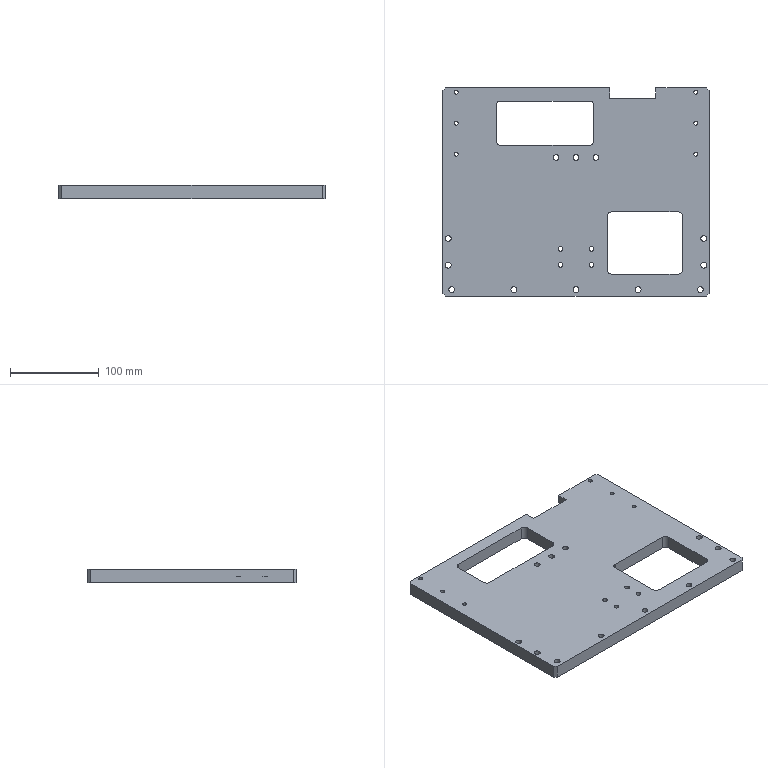Part | NX | 1 solid | 100 faces | box 300 x 235 x 15 mm | volume 860030 mm3 | cylinder 54 | plane 44 | cone 2 | commonest cylinder face diameters 10 x12 11 x12 6.6 x9 4.5 x6 8 x6 5.5 x4